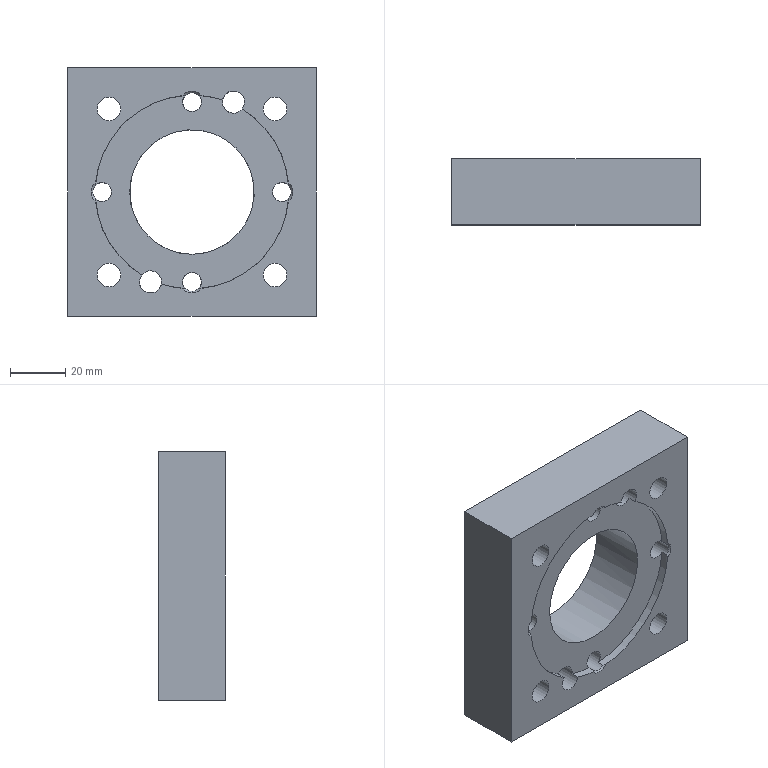Part | STEP file | 冲床-300配套压波_id958_x_t | 1 solid | 40 faces | box 90 x 24 x 90 mm | volume 133155 mm3 | cylinder 21 | plane 11 | cone 8 | commonest cylinder face diameters 70 x6 6.8 x4 8.5 x4 14 x4 8 x2 45 x1
STEP:
#1=CARTESIAN_POINT('',(1380.937,43.5,46.878));
#2=VERTEX_POINT('',#1);
#3=CARTESIAN_POINT('',(1380.937,46.5,46.878));
#4=VERTEX_POINT('',#3);
#5=CARTESIAN_POINT('',(1380.937,20.,46.878));
#6=DIRECTION('',(0.,1.,0.));
#7=VECTOR('',#6,1.);
#8=LINE('',#5,#7);
#9=EDGE_CURVE('',#2,#4,#8,.T.);
#10=ORIENTED_EDGE('',*,*,#9,.F.);
#11=CARTESIAN_POINT('',(1388.763,43.5,45.233));
#12=VERTEX_POINT('',#11);
#13=CARTESIAN_POINT('',(1392.,43.5,80.083));
#14=DIRECTION('',(0.,-1.,0.));
#15=DIRECTION('',(0.,0.,-1.));
#16=AXIS2_PLACEMENT_3D('',#13,#14,#15);
#17=CIRCLE('',#16,35.);
#18=EDGE_CURVE('',#2,#12,#17,.T.);
#19=ORIENTED_EDGE('',*,*,#18,.T.);
#20=CARTESIAN_POINT('',(1389.61,44.1,45.165));
#21=VERTEX_POINT('',#20);
#22=CARTESIAN_POINT('',(1388.763,43.5,45.233));
#23=CARTESIAN_POINT('',(1389.039,43.708,45.208));
#24=CARTESIAN_POINT('',(1389.32,43.91,45.185));
#25=CARTESIAN_POINT('',(1389.61,44.1,45.165));
#26=B_SPLINE_CURVE_WITH_KNOTS('',3,(#22,#23,#24,#25),.UNSPECIFIED.,.F.,.F.,(4,4),(0.,1.),.UNSPECIFIED.);
#27=EDGE_CURVE('',#12,#21,#26,.T.);
#28=ORIENTED_EDGE('',*,*,#27,.T.);
#29=CARTESIAN_POINT('',(1389.61,46.5,45.165));
#30=VERTEX_POINT('',#29);
#31=CARTESIAN_POINT('',(1389.61,-247465.249,45.165));
#32=DIRECTION('',(0.,1.,0.));
#33=VECTOR('',#32,1.);
#34=LINE('',#31,#33);
#35=EDGE_CURVE('',#21,#30,#34,.T.);
#36=ORIENTED_EDGE('',*,*,#35,.T.);
#37=CARTESIAN_POINT('',(1392.,46.5,80.083));
#38=DIRECTION('',(0.,1.,0.));
#39=DIRECTION('',(-1.,0.,0.));
#40=AXIS2_PLACEMENT_3D('',#37,#38,#39);
#41=CIRCLE('',#40,35.);
#42=EDGE_CURVE('',#30,#4,#41,.T.);
#43=ORIENTED_EDGE('',*,*,#42,.T.);
#44=EDGE_LOOP('',(#10,#19,#28,#36,#43));
#45=FACE_OUTER_BOUND('',#44,.T.);
#46=CARTESIAN_POINT('',(1392.,-46.,80.083));
#47=DIRECTION('',(0.,-1.,0.));
#48=DIRECTION('',(0.,0.,-1.));
#49=AXIS2_PLACEMENT_3D('',#46,#47,#48);
#50=CYLINDRICAL_SURFACE('',#49,35.);
#51=ADVANCED_FACE('',(#45),#50,.F.);
#52=CARTESIAN_POINT('',(1373.909,46.5,50.122));
#53=VERTEX_POINT('',#52);
#54=CARTESIAN_POINT('',(1373.909,43.5,50.122));
#55=VERTEX_POINT('',#54);
#56=CARTESIAN_POINT('',(1373.909,20.,50.122));
#57=DIRECTION('',(0.,-1.,0.));
#58=VECTOR('',#57,1.);
#59=LINE('',#56,#58);
#60=EDGE_CURVE('',#53,#55,#59,.T.);
#61=ORIENTED_EDGE('',*,*,#60,.F.);
#62=CARTESIAN_POINT('',(1357.082,46.5,77.694));
#63=VERTEX_POINT('',#62);
#64=CARTESIAN_POINT('',(1392.,46.5,80.083));
#65=DIRECTION('',(0.,1.,0.));
#66=DIRECTION('',(-1.,0.,0.));
#67=AXIS2_PLACEMENT_3D('',#64,#65,#66);
#68=CIRCLE('',#67,35.);
#69=EDGE_CURVE('',#53,#63,#68,.T.);
#70=ORIENTED_EDGE('',*,*,#69,.T.);
#71=CARTESIAN_POINT('',(1357.082,44.1,77.694));
#72=VERTEX_POINT('',#71);
#73=CARTESIAN_POINT('',(1357.082,-247465.293,77.694));
#74=DIRECTION('',(0.,-1.,0.));
#75=VECTOR('',#74,1.);
#76=LINE('',#73,#75);
#77=EDGE_CURVE('',#63,#72,#76,.T.);
#78=ORIENTED_EDGE('',*,*,#77,.T.);
#79=CARTESIAN_POINT('',(1357.15,43.5,76.847));
#80=VERTEX_POINT('',#79);
#81=CARTESIAN_POINT('',(1357.082,44.1,77.694));
#82=CARTESIAN_POINT('',(1357.102,43.91,77.404));
#83=CARTESIAN_POINT('',(1357.124,43.708,77.123));
#84=CARTESIAN_POINT('',(1357.15,43.5,76.847));
#85=B_SPLINE_CURVE_WITH_KNOTS('',3,(#81,#82,#83,#84),.UNSPECIFIED.,.F.,.F.,(4,4),(0.,1.),.UNSPECIFIED.);
#86=EDGE_CURVE('',#72,#80,#85,.T.);
#87=ORIENTED_EDGE('',*,*,#86,.T.);
#88=CARTESIAN_POINT('',(1392.,43.5,80.083));
#89=DIRECTION('',(0.,-1.,0.));
#90=DIRECTION('',(0.,0.,-1.));
#91=AXIS2_PLACEMENT_3D('',#88,#89,#90);
#92=CIRCLE('',#91,35.);
#93=EDGE_CURVE('',#80,#55,#92,.T.);
#94=ORIENTED_EDGE('',*,*,#93,.T.);
#95=EDGE_LOOP('',(#61,#70,#78,#87,#94));
#96=FACE_OUTER_BOUND('',#95,.T.);
#97=CARTESIAN_POINT('',(1392.,-46.,80.083));
#98=DIRECTION('',(0.,-1.,0.));
#99=DIRECTION('',(0.,0.,-1.));
#100=AXIS2_PLACEMENT_3D('',#97,#98,#99);
#101=CYLINDRICAL_SURFACE('',#100,35.);
#102=ADVANCED_FACE('',(#96),#101,.F.);
#103=CARTESIAN_POINT('',(1403.063,43.5,113.289));
#104=VERTEX_POINT('',#103);
#105=CARTESIAN_POINT('',(1403.063,46.5,113.289));
#106=VERTEX_POINT('',#105);
#107=CARTESIAN_POINT('',(1403.063,20.,113.289));
#108=DIRECTION('',(0.,1.,0.));
#109=VECTOR('',#108,1.);
#110=LINE('',#107,#109);
#111=EDGE_CURVE('',#104,#106,#110,.T.);
#112=ORIENTED_EDGE('',*,*,#111,.F.);
#113=CARTESIAN_POINT('',(1395.237,43.5,114.933));
#114=VERTEX_POINT('',#113);
#115=CARTESIAN_POINT('',(1392.,43.5,80.083));
#116=DIRECTION('',(0.,-1.,0.));
#117=DIRECTION('',(0.,0.,-1.));
#118=AXIS2_PLACEMENT_3D('',#115,#116,#117);
#119=CIRCLE('',#118,35.);
#120=EDGE_CURVE('',#104,#114,#119,.T.);
#121=ORIENTED_EDGE('',*,*,#120,.T.);
#122=CARTESIAN_POINT('',(1394.39,44.1,115.002));
#123=VERTEX_POINT('',#122);
#124=CARTESIAN_POINT('',(1395.237,43.5,114.933));
#125=CARTESIAN_POINT('',(1394.961,43.708,114.959));
#126=CARTESIAN_POINT('',(1394.68,43.91,114.982));
#127=CARTESIAN_POINT('',(1394.39,44.1,115.002));
#128=B_SPLINE_CURVE_WITH_KNOTS('',3,(#124,#125,#126,#127),.UNSPECIFIED.,.F.,.F.,(4,4),(0.,1.),.UNSPECIFIED.);
#129=EDGE_CURVE('',#114,#123,#128,.T.);
#130=ORIENTED_EDGE('',*,*,#129,.T.);
#131=CARTESIAN_POINT('',(1394.39,46.5,115.002));
#132=VERTEX_POINT('',#131);
#133=CARTESIAN_POINT('',(1394.39,-247465.244,115.002));
#134=DIRECTION('',(0.,1.,0.));
#135=VECTOR('',#134,1.);
#136=LINE('',#133,#135);
#137=EDGE_CURVE('',#123,#132,#136,.T.);
#138=ORIENTED_EDGE('',*,*,#137,.T.);
#139=CARTESIAN_POINT('',(1392.,46.5,80.083));
#140=DIRECTION('',(0.,1.,0.));
#141=DIRECTION('',(-1.,0.,0.));
#142=AXIS2_PLACEMENT_3D('',#139,#140,#141);
#143=CIRCLE('',#142,35.);
#144=EDGE_CURVE('',#132,#106,#143,.T.);
#145=ORIENTED_EDGE('',*,*,#144,.T.);
#146=EDGE_LOOP('',(#112,#121,#130,#138,#145));
#147=FACE_OUTER_BOUND('',#146,.T.);
#148=CARTESIAN_POINT('',(1392.,-46.,80.083));
#149=DIRECTION('',(0.,-1.,0.));
#150=DIRECTION('',(0.,0.,-1.));
#151=AXIS2_PLACEMENT_3D('',#148,#149,#150);
#152=CYLINDRICAL_SURFACE('',#151,35.);
#153=ADVANCED_FACE('',(#147),#152,.F.);
#154=CARTESIAN_POINT('',(1410.091,46.5,110.045));
#155=VERTEX_POINT('',#154);
#156=CARTESIAN_POINT('',(1410.091,43.5,110.045));
#157=VERTEX_POINT('',#156);
#158=CARTESIAN_POINT('',(1410.091,20.,110.045));
#159=DIRECTION('',(0.,-1.,0.));
#160=VECTOR('',#159,1.);
#161=LINE('',#158,#160);
#162=EDGE_CURVE('',#155,#157,#161,.T.);
#163=ORIENTED_EDGE('',*,*,#162,.F.);
#164=CARTESIAN_POINT('',(1426.918,46.5,82.473));
#165=VERTEX_POINT('',#164);
#166=CARTESIAN_POINT('',(1392.,46.5,80.083));
#167=DIRECTION('',(0.,1.,0.));
#168=DIRECTION('',(-1.,0.,0.));
#169=AXIS2_PLACEMENT_3D('',#166,#167,#168);
#170=CIRCLE('',#169,35.);
#171=EDGE_CURVE('',#155,#165,#170,.T.);
#172=ORIENTED_EDGE('',*,*,#171,.T.);
#173=CARTESIAN_POINT('',(1426.918,44.1,82.473));
#174=VERTEX_POINT('',#173);
#175=CARTESIAN_POINT('',(1426.918,-247465.2,82.473));
#176=DIRECTION('',(0.,-1.,0.));
#177=VECTOR('',#176,1.);
#178=LINE('',#175,#177);
#179=EDGE_CURVE('',#165,#174,#178,.T.);
#180=ORIENTED_EDGE('',*,*,#179,.T.);
#181=CARTESIAN_POINT('',(1426.85,43.5,83.32));
#182=VERTEX_POINT('',#181);
#183=CARTESIAN_POINT('',(1426.918,44.1,82.473));
#184=CARTESIAN_POINT('',(1426.898,43.91,82.763));
#185=CARTESIAN_POINT('',(1426.876,43.708,83.044));
#186=CARTESIAN_POINT('',(1426.85,43.5,83.32));
#187=B_SPLINE_CURVE_WITH_KNOTS('',3,(#183,#184,#185,#186),.UNSPECIFIED.,.F.,.F.,(4,4),(0.,1.),.UNSPECIFIED.);
#188=EDGE_CURVE('',#174,#182,#187,.T.);
#189=ORIENTED_EDGE('',*,*,#188,.T.);
#190=CARTESIAN_POINT('',(1392.,43.5,80.083));
#191=DIRECTION('',(0.,-1.,0.));
#192=DIRECTION('',(0.,0.,-1.));
#193=AXIS2_PLACEMENT_3D('',#190,#191,#192);
#194=CIRCLE('',#193,35.);
#195=EDGE_CURVE('',#182,#157,#194,.T.);
#196=ORIENTED_EDGE('',*,*,#195,.T.);
#197=EDGE_LOOP('',(#163,#172,#180,#189,#196));
#198=FACE_OUTER_BOUND('',#197,.T.);
#199=CARTESIAN_POINT('',(1392.,-46.,80.083));
#200=DIRECTION('',(0.,-1.,0.));
#201=DIRECTION('',(0.,0.,-1.));
#202=AXIS2_PLACEMENT_3D('',#199,#200,#201);
#203=CYLINDRICAL_SURFACE('',#202,35.);
#204=ADVANCED_FACE('',(#198),#203,.F.);
#205=CARTESIAN_POINT('',(1357.082,44.1,82.473));
#206=VERTEX_POINT('',#205);
#207=CARTESIAN_POINT('',(1357.082,46.5,82.473));
#208=VERTEX_POINT('',#207);
#209=CARTESIAN_POINT('',(1357.082,-247465.293,82.473));
#210=DIRECTION('',(0.,1.,0.));
#211=VECTOR('',#210,1.);
#212=LINE('',#209,#211);
#213=EDGE_CURVE('',#206,#208,#212,.T.);
#214=ORIENTED_EDGE('',*,*,#213,.T.);
#215=CARTESIAN_POINT('',(1389.61,46.5,115.002));
#216=VERTEX_POINT('',#215);
#217=CARTESIAN_POINT('',(1392.,46.5,80.083));
#218=DIRECTION('',(0.,1.,0.));
#219=DIRECTION('',(-1.,0.,0.));
#220=AXIS2_PLACEMENT_3D('',#217,#218,#219);
#221=CIRCLE('',#220,35.);
#222=EDGE_CURVE('',#208,#216,#221,.T.);
#223=ORIENTED_EDGE('',*,*,#222,.T.);
#224=CARTESIAN_POINT('',(1389.61,44.1,115.002));
#225=VERTEX_POINT('',#224);
#226=CARTESIAN_POINT('',(1389.61,-247465.244,115.002));
#227=DIRECTION('',(0.,-1.,0.));
#228=VECTOR('',#227,1.);
#229=LINE('',#226,#228);
#230=EDGE_CURVE('',#216,#225,#229,.T.);
#231=ORIENTED_EDGE('',*,*,#230,.T.);
#232=CARTESIAN_POINT('',(1388.763,43.5,114.933));
#233=VERTEX_POINT('',#232);
#234=CARTESIAN_POINT('',(1389.61,44.1,115.002));
#235=CARTESIAN_POINT('',(1389.32,43.91,114.982));
#236=CARTESIAN_POINT('',(1389.039,43.708,114.959));
#237=CARTESIAN_POINT('',(1388.763,43.5,114.933));
#238=B_SPLINE_CURVE_WITH_KNOTS('',3,(#234,#235,#236,#237),.UNSPECIFIED.,.F.,.F.,(4,4),(0.,1.),.UNSPECIFIED.);
#239=EDGE_CURVE('',#225,#233,#238,.T.);
#240=ORIENTED_EDGE('',*,*,#239,.T.);
#241=CARTESIAN_POINT('',(1357.15,43.5,83.32));
#242=VERTEX_POINT('',#241);
#243=CARTESIAN_POINT('',(1392.,43.5,80.083));
#244=DIRECTION('',(0.,-1.,0.));
#245=DIRECTION('',(0.,0.,-1.));
#246=AXIS2_PLACEMENT_3D('',#243,#244,#245);
#247=CIRCLE('',#246,35.);
#248=EDGE_CURVE('',#233,#242,#247,.T.);
#249=ORIENTED_EDGE('',*,*,#248,.T.);
#250=CARTESIAN_POINT('',(1357.15,43.5,83.32));
#251=CARTESIAN_POINT('',(1357.124,43.708,83.044));
#252=CARTESIAN_POINT('',(1357.102,43.91,82.763));
#253=CARTESIAN_POINT('',(1357.082,44.1,82.473));
#254=B_SPLINE_CURVE_WITH_KNOTS('',3,(#250,#251,#252,#253),.UNSPECIFIED.,.F.,.F.,(4,4),(0.,1.),.UNSPECIFIED.);
#255=EDGE_CURVE('',#242,#206,#254,.T.);
#256=ORIENTED_EDGE('',*,*,#255,.T.);
#257=EDGE_LOOP('',(#214,#223,#231,#240,#249,#256));
#258=FACE_OUTER_BOUND('',#257,.T.);
#259=CARTESIAN_POINT('',(1392.,-46.,80.083));
#260=DIRECTION('',(0.,-1.,0.));
#261=DIRECTION('',(0.,0.,-1.));
#262=AXIS2_PLACEMENT_3D('',#259,#260,#261);
#263=CYLINDRICAL_SURFACE('',#262,35.);
#264=ADVANCED_FACE('',(#258),#263,.F.);
#265=CARTESIAN_POINT('',(1395.237,43.5,45.233));
#266=VERTEX_POINT('',#265);
#267=CARTESIAN_POINT('',(1426.85,43.5,76.847));
#268=VERTEX_POINT('',#267);
#269=CARTESIAN_POINT('',(1392.,43.5,80.083));
#270=DIRECTION('',(0.,-1.,0.));
#271=DIRECTION('',(0.,0.,-1.));
#272=AXIS2_PLACEMENT_3D('',#269,#270,#271);
#273=CIRCLE('',#272,35.);
#274=EDGE_CURVE('',#266,#268,#273,.T.);
#275=ORIENTED_EDGE('',*,*,#274,.T.);
#276=CARTESIAN_POINT('',(1426.918,44.1,77.694));
#277=VERTEX_POINT('',#276);
#278=CARTESIAN_POINT('',(1426.85,43.5,76.847));
#279=CARTESIAN_POINT('',(1426.876,43.708,77.123));
#280=CARTESIAN_POINT('',(1426.898,43.91,77.404));
#281=CARTESIAN_POINT('',(1426.918,44.1,77.694));
#282=B_SPLINE_CURVE_WITH_KNOTS('',3,(#278,#279,#280,#281),.UNSPECIFIED.,.F.,.F.,(4,4),(0.,1.),.UNSPECIFIED.);
#283=EDGE_CURVE('',#268,#277,#282,.T.);
#284=ORIENTED_EDGE('',*,*,#283,.T.);
#285=CARTESIAN_POINT('',(1426.918,46.5,77.694));
#286=VERTEX_POINT('',#285);
#287=CARTESIAN_POINT('',(1426.918,-247465.2,77.694));
#288=DIRECTION('',(0.,1.,0.));
#289=VECTOR('',#288,1.);
#290=LINE('',#287,#289);
#291=EDGE_CURVE('',#277,#286,#290,.T.);
#292=ORIENTED_EDGE('',*,*,#291,.T.);
#293=CARTESIAN_POINT('',(1394.39,46.5,45.165));
#294=VERTEX_POINT('',#293);
#295=CARTESIAN_POINT('',(1392.,46.5,80.083));
#296=DIRECTION('',(0.,1.,0.));
#297=DIRECTION('',(-1.,0.,0.));
#298=AXIS2_PLACEMENT_3D('',#295,#296,#297);
#299=CIRCLE('',#298,35.);
#300=EDGE_CURVE('',#286,#294,#299,.T.);
#301=ORIENTED_EDGE('',*,*,#300,.T.);
#302=CARTESIAN_POINT('',(1394.39,44.1,45.165));
#303=VERTEX_POINT('',#302);
#304=CARTESIAN_POINT('',(1394.39,-247465.249,45.165));
#305=DIRECTION('',(0.,-1.,0.));
#306=VECTOR('',#305,1.);
#307=LINE('',#304,#306);
#308=EDGE_CURVE('',#294,#303,#307,.T.);
#309=ORIENTED_EDGE('',*,*,#308,.T.);
#310=CARTESIAN_POINT('',(1394.39,44.1,45.165));
#311=CARTESIAN_POINT('',(1394.68,43.91,45.185));
#312=CARTESIAN_POINT('',(1394.961,43.708,45.208));
#313=CARTESIAN_POINT('',(1395.237,43.5,45.233));
#314=B_SPLINE_CURVE_WITH_KNOTS('',3,(#310,#311,#312,#313),.UNSPECIFIED.,.F.,.F.,(4,4),(0.,1.),.UNSPECIFIED.);
#315=EDGE_CURVE('',#303,#266,#314,.T.);
#316=ORIENTED_EDGE('',*,*,#315,.T.);
#317=EDGE_LOOP('',(#275,#284,#292,#301,#309,#316));
#318=FACE_OUTER_BOUND('',#317,.T.);
#319=CARTESIAN_POINT('',(1392.,-46.,80.083));
#320=DIRECTION('',(0.,-1.,0.));
#321=DIRECTION('',(0.,0.,-1.));
#322=AXIS2_PLACEMENT_3D('',#319,#320,#321);
#323=CYLINDRICAL_SURFACE('',#322,35.);
#324=ADVANCED_FACE('',(#318),#323,.F.);
#325=CARTESIAN_POINT('',(1403.,67.5,112.583));
#326=VERTEX_POINT('',#325);
#327=CARTESIAN_POINT('',(1407.,67.5,112.583));
#328=DIRECTION('',(0.,-1.,0.));
#329=DIRECTION('',(-1.,0.,0.));
#330=AXIS2_PLACEMENT_3D('',#327,#328,#329);
#331=CIRCLE('',#330,4.);
#332=EDGE_CURVE('',#326,#326,#331,.T.);
#333=ORIENTED_EDGE('',*,*,#332,.T.);
#334=EDGE_LOOP('',(#333));
#335=FACE_BOUND('',#334,.T.);
#336=CARTESIAN_POINT('',(1373.,67.5,47.583));
#337=VERTEX_POINT('',#336);
#338=CARTESIAN_POINT('',(1377.,67.5,47.583));
#339=DIRECTION('',(0.,-1.,0.));
#340=DIRECTION('',(-1.,0.,0.));
#341=AXIS2_PLACEMENT_3D('',#338,#339,#340);
#342=CIRCLE('',#341,4.);
#343=EDGE_CURVE('',#337,#337,#342,.T.);
#344=ORIENTED_EDGE('',*,*,#343,.T.);
#345=EDGE_LOOP('',(#344));
#346=FACE_BOUND('',#345,.T.);
#347=CARTESIAN_POINT('',(1392.,67.5,43.583));
#348=VERTEX_POINT('',#347);
#349=CARTESIAN_POINT('',(1392.,67.5,47.583));
#350=DIRECTION('',(0.,-1.,0.));
#351=DIRECTION('',(0.,0.,-1.));
#352=AXIS2_PLACEMENT_3D('',#349,#350,#351);
#353=CIRCLE('',#352,4.);
#354=EDGE_CURVE('',#348,#348,#353,.T.);
#355=ORIENTED_EDGE('',*,*,#354,.T.);
#356=EDGE_LOOP('',(#355));
#357=FACE_BOUND('',#356,.T.);
#358=CARTESIAN_POINT('',(1424.5,67.5,76.083));
#359=VERTEX_POINT('',#358);
#360=CARTESIAN_POINT('',(1424.5,67.5,80.083));
#361=DIRECTION('',(0.,-1.,0.));
#362=DIRECTION('',(0.,0.,-1.));
#363=AXIS2_PLACEMENT_3D('',#360,#361,#362);
#364=CIRCLE('',#363,4.);
#365=EDGE_CURVE('',#359,#359,#364,.T.);
#366=ORIENTED_EDGE('',*,*,#365,.T.);
#367=EDGE_LOOP('',(#366));
#368=FACE_BOUND('',#367,.T.);
#369=CARTESIAN_POINT('',(1359.5,67.5,76.083));
#370=VERTEX_POINT('',#369);
#371=CARTESIAN_POINT('',(1359.5,67.5,80.083));
#372=DIRECTION('',(0.,-1.,0.));
#373=DIRECTION('',(0.,0.,-1.));
#374=AXIS2_PLACEMENT_3D('',#371,#372,#373);
#375=CIRCLE('',#374,4.);
#376=EDGE_CURVE('',#370,#370,#375,.T.);
#377=ORIENTED_EDGE('',*,*,#376,.T.);
#378=EDGE_LOOP('',(#377));
#379=FACE_BOUND('',#378,.T.);
#380=CARTESIAN_POINT('',(1392.,67.5,108.583));
#381=VERTEX_POINT('',#380);
#382=CARTESIAN_POINT('',(1392.,67.5,112.583));
#383=DIRECTION('',(0.,-1.,0.));
#384=DIRECTION('',(0.,0.,-1.));
#385=AXIS2_PLACEMENT_3D('',#382,#383,#384);
#386=CIRCLE('',#385,4.);
#387=EDGE_CURVE('',#381,#381,#386,.T.);
#388=ORIENTED_EDGE('',*,*,#387,.T.);
#389=EDGE_LOOP('',(#388));
#390=FACE_BOUND('',#389,.T.);
#391=CARTESIAN_POINT('',(1392.,67.5,57.583));
#392=VERTEX_POINT('',#391);
#393=CARTESIAN_POINT('',(1392.,67.5,80.083));
#394=DIRECTION('',(0.,1.,0.));
#395=DIRECTION('',(0.,0.,-1.));
#396=AXIS2_PLACEMENT_3D('',#393,#394,#395);
#397=CIRCLE('',#396,22.5);
#398=EDGE_CURVE('',#392,#392,#397,.T.);
#399=ORIENTED_EDGE('',*,*,#398,.F.);
#400=EDGE_LOOP('',(#399));
#401=FACE_BOUND('',#400,.T.);
#402=CARTESIAN_POINT('',(1422.052,67.5,103.136));
#403=VERTEX_POINT('',#402);
#404=CARTESIAN_POINT('',(1422.052,67.5,110.136));
#405=DIRECTION('',(0.,1.,0.));
#406=DIRECTION('',(0.,0.,-1.));
#407=AXIS2_PLACEMENT_3D('',#404,#405,#406);
#408=CIRCLE('',#407,7.);
#409=EDGE_CURVE('',#403,#403,#408,.T.);
#410=ORIENTED_EDGE('',*,*,#409,.F.);
#411=EDGE_LOOP('',(#410));
#412=FACE_BOUND('',#411,.T.);
#413=CARTESIAN_POINT('',(1361.948,67.5,43.031));
#414=VERTEX_POINT('',#413);
#415=CARTESIAN_POINT('',(1361.948,67.5,50.031));
#416=DIRECTION('',(0.,1.,0.));
#417=DIRECTION('',(0.,0.,-1.));
#418=AXIS2_PLACEMENT_3D('',#415,#416,#417);
#419=CIRCLE('',#418,7.);
#420=EDGE_CURVE('',#414,#414,#419,.T.);
#421=ORIENTED_EDGE('',*,*,#420,.F.);
#422=EDGE_LOOP('',(#421));
#423=FACE_BOUND('',#422,.T.);
#424=CARTESIAN_POINT('',(1422.052,67.5,43.031));
#425=VERTEX_POINT('',#424);
#426=CARTESIAN_POINT('',(1422.052,67.5,50.031));
#427=DIRECTION('',(0.,1.,0.));
#428=DIRECTION('',(0.,0.,-1.));
#429=AXIS2_PLACEMENT_3D('',#426,#427,#428);
#430=CIRCLE('',#429,7.);
#431=EDGE_CURVE('',#425,#425,#430,.T.);
#432=ORIENTED_EDGE('',*,*,#431,.F.);
#433=EDGE_LOOP('',(#432));
#434=FACE_BOUND('',#433,.T.);
#435=CARTESIAN_POINT('',(1361.948,67.5,103.136));
#436=VERTEX_POINT('',#435);
#437=CARTESIAN_POINT('',(1361.948,67.5,110.136));
#438=DIRECTION('',(0.,-1.,0.));
#439=DIRECTION('',(0.,0.,-1.));
#440=AXIS2_PLACEMENT_3D('',#437,#438,#439);
#441=CIRCLE('',#440,7.);
#442=EDGE_CURVE('',#436,#436,#441,.T.);
#443=ORIENTED_EDGE('',*,*,#442,.T.);
#444=EDGE_LOOP('',(#443));
#445=FACE_BOUND('',#444,.T.);
#446=CARTESIAN_POINT('',(1347.,67.5,35.083));
#447=VERTEX_POINT('',#446);
#448=CARTESIAN_POINT('',(1347.,67.5,125.083));
#449=VERTEX_POINT('',#448);
#450=CARTESIAN_POINT('',(1347.,67.5,24.7));
#451=DIRECTION('',(0.,0.,1.));
#452=VECTOR('',#451,1.);
#453=LINE('',#450,#452);
#454=EDGE_CURVE('',#447,#449,#453,.T.);
#455=ORIENTED_EDGE('',*,*,#454,.T.);
#456=CARTESIAN_POINT('',(1437.,67.5,125.083));
#457=VERTEX_POINT('',#456);
#458=CARTESIAN_POINT('',(1437.,67.5,125.083));
#459=DIRECTION('',(1.,0.,0.));
#460=VECTOR('',#459,1.);
#461=LINE('',#458,#460);
#462=EDGE_CURVE('',#449,#457,#461,.T.);
#463=ORIENTED_EDGE('',*,*,#462,.T.);
#464=CARTESIAN_POINT('',(1437.,67.5,35.083));
#465=VERTEX_POINT('',#464);
#466=CARTESIAN_POINT('',(1437.,67.5,35.083));
#467=DIRECTION('',(0.,0.,-1.));
#468=VECTOR('',#467,1.);
#469=LINE('',#466,#468);
#470=EDGE_CURVE('',#457,#465,#469,.T.);
#471=ORIENTED_EDGE('',*,*,#470,.T.);
#472=CARTESIAN_POINT('',(1347.,67.5,35.083));
#473=DIRECTION('',(-1.,0.,0.));
#474=VECTOR('',#473,1.);
#475=LINE('',#472,#474);
#476=EDGE_CURVE('',#465,#447,#475,.T.);
#477=ORIENTED_EDGE('',*,*,#476,.T.);
#478=EDGE_LOOP('',(#455,#463,#471,#477));
#479=FACE_BOUND('',#478,.T.);
#480=CARTESIAN_POINT('',(-14.812,67.5,1.089));
#481=DIRECTION('',(0.,1.,0.));
#482=DIRECTION('',(0.,0.,-1.));
#483=AXIS2_PLACEMENT_3D('',#480,#481,#482);
#484=PLANE('',#483);
#485=ADVANCED_FACE('',(#335,#346,#357,#368,#379,#390,#401,#412,#423,#434,#445,#479),#484,.T.);
#486=CARTESIAN_POINT('',(1361.948,43.5,45.781));
#487=VERTEX_POINT('',#486);
#488=CARTESIAN_POINT('',(1361.948,43.5,50.031));
#489=DIRECTION('',(0.,1.,0.));
#490=DIRECTION('',(0.,0.,-1.));
#491=AXIS2_PLACEMENT_3D('',#488,#489,#490);
#492=CIRCLE('',#491,4.25);
#493=EDGE_CURVE('',#487,#487,#492,.T.);
#494=ORIENTED_EDGE('',*,*,#493,.F.);
#495=EDGE_LOOP('',(#494));
#496=FACE_BOUND('',#495,.T.);
#497=CARTESIAN_POINT('',(1361.948,53.5,45.781));
#498=VERTEX_POINT('',#497);
#499=CARTESIAN_POINT('',(1361.948,53.5,50.031));
#500=DIRECTION('',(0.,-1.,0.));
#501=DIRECTION('',(0.,0.,-1.));
#502=AXIS2_PLACEMENT_3D('',#499,#500,#501);
#503=CIRCLE('',#502,4.25);
#504=EDGE_CURVE('',#498,#498,#503,.T.);
#505=ORIENTED_EDGE('',*,*,#504,.F.);
#506=EDGE_LOOP('',(#505));
#507=FACE_BOUND('',#506,.T.);
#508=CARTESIAN_POINT('',(1361.948,23.5,50.031));
#509=DIRECTION('',(0.,1.,0.));
#510=DIRECTION('',(1.,0.,0.));
#511=AXIS2_PLACEMENT_3D('',#508,#509,#510);
#512=CYLINDRICAL_SURFACE('',#511,4.25);
#513=ADVANCED_FACE('',(#496,#507),#512,.F.);
#514=CARTESIAN_POINT('',(1422.052,43.5,105.886));
#515=VERTEX_POINT('',#514);
#516=CARTESIAN_POINT('',(1422.052,43.5,110.136));
#517=DIRECTION('',(0.,1.,0.));
#518=DIRECTION('',(0.,0.,-1.));
#519=AXIS2_PLACEMENT_3D('',#516,#517,#518);
#520=CIRCLE('',#519,4.25);
#521=EDGE_CURVE('',#515,#515,#520,.T.);
#522=ORIENTED_EDGE('',*,*,#521,.F.);
#523=EDGE_LOOP('',(#522));
#524=FACE_BOUND('',#523,.T.);
#525=CARTESIAN_POINT('',(1422.052,53.5,105.886));
#526=VERTEX_POINT('',#525);
#527=CARTESIAN_POINT('',(1422.052,53.5,110.136));
#528=DIRECTION('',(0.,-1.,0.));
#529=DIRECTION('',(0.,0.,-1.));
#530=AXIS2_PLACEMENT_3D('',#527,#528,#529);
#531=CIRCLE('',#530,4.25);
#532=EDGE_CURVE('',#526,#526,#531,.T.);
#533=ORIENTED_EDGE('',*,*,#532,.F.);
#534=EDGE_LOOP('',(#533));
#535=FACE_BOUND('',#534,.T.);
#536=CARTESIAN_POINT('',(1422.052,23.5,110.136));
#537=DIRECTION('',(0.,1.,0.));
#538=DIRECTION('',(1.,0.,0.));
#539=AXIS2_PLACEMENT_3D('',#536,#537,#538);
#540=CYLINDRICAL_SURFACE('',#539,4.25);
#541=ADVANCED_FACE('',(#524,#535),#540,.F.);
#542=CARTESIAN_POINT('',(1422.052,43.5,45.781));
#543=VERTEX_POINT('',#542);
#544=CARTESIAN_POINT('',(1422.052,43.5,50.031));
#545=DIRECTION('',(0.,1.,0.));
#546=DIRECTION('',(0.,0.,-1.));
#547=AXIS2_PLACEMENT_3D('',#544,#545,#546);
#548=CIRCLE('',#547,4.25);
#549=EDGE_CURVE('',#543,#543,#548,.T.);
#550=ORIENTED_EDGE('',*,*,#549,.F.);
#551=EDGE_LOOP('',(#550));
#552=FACE_BOUND('',#551,.T.);
#553=CARTESIAN_POINT('',(1422.052,53.5,45.781));
#554=VERTEX_POINT('',#553);
#555=CARTESIAN_POINT('',(1422.052,53.5,50.031));
#556=DIRECTION('',(0.,-1.,0.));
#557=DIRECTION('',(0.,0.,-1.));
#558=AXIS2_PLACEMENT_3D('',#555,#556,#557);
#559=CIRCLE('',#558,4.25);
#560=EDGE_CURVE('',#554,#554,#559,.T.);
#561=ORIENTED_EDGE('',*,*,#560,.F.);
#562=EDGE_LOOP('',(#561));
#563=FACE_BOUND('',#562,.T.);
#564=CARTESIAN_POINT('',(1422.052,23.5,50.031));
#565=DIRECTION('',(0.,1.,0.));
#566=DIRECTION('',(1.,0.,0.));
#567=AXIS2_PLACEMENT_3D('',#564,#565,#566);
#568=CYLINDRICAL_SURFACE('',#567,4.25);
#569=ADVANCED_FACE('',(#552,#563),#568,.F.);
#570=CARTESIAN_POINT('',(1407.,43.5,112.583));
#571=DIRECTION('',(0.,-1.,0.));
#572=DIRECTION('',(-1.,0.,0.));
#573=AXIS2_PLACEMENT_3D('',#570,#571,#572);
#574=CIRCLE('',#573,4.);
#575=EDGE_CURVE('',#157,#104,#574,.T.);
#576=ORIENTED_EDGE('',*,*,#575,.F.);
#577=ORIENTED_EDGE('',*,*,#195,.F.);
#578=CARTESIAN_POINT('',(1424.5,43.5,80.083));
#579=DIRECTION('',(0.,1.,0.));
#580=DIRECTION('',(0.,0.,-1.));
#581=AXIS2_PLACEMENT_3D('',#578,#579,#580);
#582=CIRCLE('',#581,4.);
#583=EDGE_CURVE('',#182,#268,#582,.T.);
#584=ORIENTED_EDGE('',*,*,#583,.T.);
#585=ORIENTED_EDGE('',*,*,#274,.F.);
#586=CARTESIAN_POINT('',(1392.,43.5,47.583));
#587=DIRECTION('',(0.,1.,0.));
#588=DIRECTION('',(0.,0.,-1.));
#589=AXIS2_PLACEMENT_3D('',#586,#587,#588);
#590=CIRCLE('',#589,4.);
#591=EDGE_CURVE('',#266,#12,#590,.T.);
#592=ORIENTED_EDGE('',*,*,#591,.T.);
#593=ORIENTED_EDGE('',*,*,#18,.F.);
#594=CARTESIAN_POINT('',(1377.,43.5,47.583));
#595=DIRECTION('',(0.,-1.,0.));
#596=DIRECTION('',(-1.,0.,0.));
#597=AXIS2_PLACEMENT_3D('',#594,#595,#596);
#598=CIRCLE('',#597,4.);
#599=EDGE_CURVE('',#55,#2,#598,.T.);
#600=ORIENTED_EDGE('',*,*,#599,.F.);
#601=ORIENTED_EDGE('',*,*,#93,.F.);
#602=CARTESIAN_POINT('',(1359.5,43.5,80.083));
#603=DIRECTION('',(0.,1.,0.));
#604=DIRECTION('',(0.,0.,-1.));
#605=AXIS2_PLACEMENT_3D('',#602,#603,#604);
#606=CIRCLE('',#605,4.);
#607=EDGE_CURVE('',#80,#242,#606,.T.);
#608=ORIENTED_EDGE('',*,*,#607,.T.);
#609=ORIENTED_EDGE('',*,*,#248,.F.);
#610=CARTESIAN_POINT('',(1392.,43.5,112.583));
#611=DIRECTION('',(0.,1.,0.));
#612=DIRECTION('',(0.,0.,-1.));
#613=AXIS2_PLACEMENT_3D('',#610,#611,#612);
#614=CIRCLE('',#613,4.);
#615=EDGE_CURVE('',#233,#114,#614,.T.);
#616=ORIENTED_EDGE('',*,*,#615,.T.);
#617=ORIENTED_EDGE('',*,*,#120,.F.);
#618=EDGE_LOOP('',(#576,#577,#584,#585,#592,#593,#600,#601,#608,#609,#616,#617));
#619=FACE_BOUND('',#618,.T.);
#620=ORIENTED_EDGE('',*,*,#549,.T.);
#621=EDGE_LOOP('',(#620));
#622=FACE_BOUND('',#621,.T.);
#623=ORIENTED_EDGE('',*,*,#521,.T.);
#624=EDGE_LOOP('',(#623));
#625=FACE_BOUND('',#624,.T.);
#626=ORIENTED_EDGE('',*,*,#493,.T.);
#627=EDGE_LOOP('',(#626));
#628=FACE_BOUND('',#627,.T.);
#629=CARTESIAN_POINT('',(1437.,43.5,35.083));
#630=VERTEX_POINT('',#629);
#631=CARTESIAN_POINT('',(1347.,43.5,35.083));
#632=VERTEX_POINT('',#631);
#633=CARTESIAN_POINT('',(1347.,43.5,35.083));
#634=DIRECTION('',(-1.,0.,0.));
#635=VECTOR('',#634,1.);
#636=LINE('',#633,#635);
#637=EDGE_CURVE('',#630,#632,#636,.T.);
#638=ORIENTED_EDGE('',*,*,#637,.F.);
#639=CARTESIAN_POINT('',(1437.,43.5,125.083));
#640=VERTEX_POINT('',#639);
#641=CARTESIAN_POINT('',(1437.,43.5,35.083));
#642=DIRECTION('',(0.,0.,-1.));
#643=VECTOR('',#642,1.);
#644=LINE('',#641,#643);
#645=EDGE_CURVE('',#640,#630,#644,.T.);
#646=ORIENTED_EDGE('',*,*,#645,.F.);
#647=CARTESIAN_POINT('',(1347.,43.5,125.083));
#648=VERTEX_POINT('',#647);
#649=CARTESIAN_POINT('',(1437.,43.5,125.083));
#650=DIRECTION('',(1.,0.,0.));
#651=VECTOR('',#650,1.);
#652=LINE('',#649,#651);
#653=EDGE_CURVE('',#648,#640,#652,.T.);
#654=ORIENTED_EDGE('',*,*,#653,.F.);
#655=CARTESIAN_POINT('',(1347.,43.5,24.7));
#656=DIRECTION('',(0.,0.,1.));
#657=VECTOR('',#656,1.);
#658=LINE('',#655,#657);
#659=EDGE_CURVE('',#632,#648,#658,.T.);
#660=ORIENTED_EDGE('',*,*,#659,.F.);
#661=EDGE_LOOP('',(#638,#646,#654,#660));
#662=FACE_BOUND('',#661,.T.);
#663=CARTESIAN_POINT('',(1361.948,43.5,105.886));
#664=VERTEX_POINT('',#663);
#665=CARTESIAN_POINT('',(1361.948,43.5,110.136));
#666=DIRECTION('',(0.,-1.,0.));
#667=DIRECTION('',(0.,0.,-1.));
#668=AXIS2_PLACEMENT_3D('',#665,#666,#667);
#669=CIRCLE('',#668,4.25);
#670=EDGE_CURVE('',#664,#664,#669,.T.);
#671=ORIENTED_EDGE('',*,*,#670,.F.);
#672=EDGE_LOOP('',(#671));
#673=FACE_BOUND('',#672,.T.);
#674=CARTESIAN_POINT('',(-14.812,43.5,1.089));
#675=DIRECTION('',(0.,1.,0.));
#676=DIRECTION('',(0.,0.,-1.));
#677=AXIS2_PLACEMENT_3D('',#674,#675,#676);
#678=PLANE('',#677);
#679=ADVANCED_FACE('',(#619,#622,#625,#628,#662,#673),#678,.F.);
#680=ORIENTED_EDGE('',*,*,#659,.T.);
#681=CARTESIAN_POINT('',(1347.,71.,125.083));
#682=DIRECTION('',(0.,1.,0.));
#683=VECTOR('',#682,1.);
#684=LINE('',#681,#683);
#685=EDGE_CURVE('',#648,#449,#684,.T.);
#686=ORIENTED_EDGE('',*,*,#685,.T.);
#687=ORIENTED_EDGE('',*,*,#454,.F.);
#688=CARTESIAN_POINT('',(1347.,63.5,35.083));
#689=DIRECTION('',(0.,1.,0.));
#690=VECTOR('',#689,1.);
#691=LINE('',#688,#690);
#692=EDGE_CURVE('',#632,#447,#691,.T.);
#693=ORIENTED_EDGE('',*,*,#692,.F.);
#694=EDGE_LOOP('',(#680,#686,#687,#693));
#695=FACE_OUTER_BOUND('',#694,.T.);
#696=CARTESIAN_POINT('',(1347.,71.,24.7));
#697=DIRECTION('',(-1.,0.,0.));
#698=DIRECTION('',(0.,0.,1.));
#699=AXIS2_PLACEMENT_3D('',#696,#697,#698);
#700=PLANE('',#699);
#701=ADVANCED_FACE('',(#695),#700,.T.);
#702=ORIENTED_EDGE('',*,*,#476,.F.);
#703=CARTESIAN_POINT('',(1437.,113.5,35.083));
#704=DIRECTION('',(0.,1.,0.));
#705=VECTOR('',#704,1.);
#706=LINE('',#703,#705);
#707=EDGE_CURVE('',#630,#465,#706,.T.);
#708=ORIENTED_EDGE('',*,*,#707,.F.);
#709=ORIENTED_EDGE('',*,*,#637,.T.);
#710=ORIENTED_EDGE('',*,*,#692,.T.);
#711=EDGE_LOOP('',(#702,#708,#709,#710));
#712=FACE_OUTER_BOUND('',#711,.T.);
#713=CARTESIAN_POINT('',(1347.,63.5,35.083));
#714=DIRECTION('',(0.,0.,1.));
#715=DIRECTION('',(1.,0.,0.));
#716=AXIS2_PLACEMENT_3D('',#713,#714,#715);
#717=PLANE('',#716);
#718=ADVANCED_FACE('',(#712),#717,.F.);
#719=ORIENTED_EDGE('',*,*,#470,.F.);
#720=CARTESIAN_POINT('',(1437.,63.5,125.083));
#721=DIRECTION('',(0.,1.,0.));
#722=VECTOR('',#721,1.);
#723=LINE('',#720,#722);
#724=EDGE_CURVE('',#640,#457,#723,.T.);
#725=ORIENTED_EDGE('',*,*,#724,.F.);
#726=ORIENTED_EDGE('',*,*,#645,.T.);
#727=ORIENTED_EDGE('',*,*,#707,.T.);
#728=EDGE_LOOP('',(#719,#725,#726,#727));
#729=FACE_OUTER_BOUND('',#728,.T.);
#730=CARTESIAN_POINT('',(1437.,113.5,35.083));
#731=DIRECTION('',(1.,0.,0.));
#732=DIRECTION('',(0.,0.,1.));
#733=AXIS2_PLACEMENT_3D('',#730,#731,#732);
#734=PLANE('',#733);
#735=ADVANCED_FACE('',(#729),#734,.T.);
#736=ORIENTED_EDGE('',*,*,#462,.F.);
#737=ORIENTED_EDGE('',*,*,#685,.F.);
#738=ORIENTED_EDGE('',*,*,#653,.T.);
#739=ORIENTED_EDGE('',*,*,#724,.T.);
#740=EDGE_LOOP('',(#736,#737,#738,#739));
#741=FACE_OUTER_BOUND('',#740,.T.);
#742=CARTESIAN_POINT('',(1437.,63.5,125.083));
#743=DIRECTION('',(0.,0.,-1.));
#744=DIRECTION('',(-1.,0.,0.));
#745=AXIS2_PLACEMENT_3D('',#742,#743,#744);
#746=PLANE('',#745);
#747=ADVANCED_FACE('',(#741),#746,.F.);
#748=CARTESIAN_POINT('',(1407.,46.5,112.583));
#749=DIRECTION('',(0.,-1.,0.));
#750=DIRECTION('',(1.,0.,0.));
#751=AXIS2_PLACEMENT_3D('',#748,#749,#750);
#752=CIRCLE('',#751,4.);
#753=EDGE_CURVE('',#106,#155,#752,.T.);
#754=ORIENTED_EDGE('',*,*,#753,.F.);
#755=ORIENTED_EDGE('',*,*,#144,.F.);
#756=CARTESIAN_POINT('',(1392.,46.5,112.583));
#757=DIRECTION('',(0.,1.,0.));
#758=DIRECTION('',(-1.,0.,0.));
#759=AXIS2_PLACEMENT_3D('',#756,#757,#758);
#760=CIRCLE('',#759,3.4);
#761=EDGE_CURVE('',#132,#216,#760,.T.);
#762=ORIENTED_EDGE('',*,*,#761,.T.);
#763=ORIENTED_EDGE('',*,*,#222,.F.);
#764=CARTESIAN_POINT('',(1359.5,46.5,80.083));
#765=DIRECTION('',(0.,1.,0.));
#766=DIRECTION('',(-1.,0.,0.));
#767=AXIS2_PLACEMENT_3D('',#764,#765,#766);
#768=CIRCLE('',#767,3.4);
#769=EDGE_CURVE('',#208,#63,#768,.T.);
#770=ORIENTED_EDGE('',*,*,#769,.T.);
#771=ORIENTED_EDGE('',*,*,#69,.F.);
#772=CARTESIAN_POINT('',(1377.,46.5,47.583));
#773=DIRECTION('',(0.,-1.,0.));
#774=DIRECTION('',(1.,0.,0.));
#775=AXIS2_PLACEMENT_3D('',#772,#773,#774);
#776=CIRCLE('',#775,4.);
#777=EDGE_CURVE('',#4,#53,#776,.T.);
#778=ORIENTED_EDGE('',*,*,#777,.F.);
#779=ORIENTED_EDGE('',*,*,#42,.F.);
#780=CARTESIAN_POINT('',(1392.,46.5,47.583));
#781=DIRECTION('',(0.,1.,0.));
#782=DIRECTION('',(-1.,0.,0.));
#783=AXIS2_PLACEMENT_3D('',#780,#781,#782);
#784=CIRCLE('',#783,3.4);
#785=EDGE_CURVE('',#30,#294,#784,.T.);
#786=ORIENTED_EDGE('',*,*,#785,.T.);
#787=ORIENTED_EDGE('',*,*,#300,.F.);
#788=CARTESIAN_POINT('',(1424.5,46.5,80.083));
#789=DIRECTION('',(0.,1.,0.));
#790=DIRECTION('',(-1.,0.,0.));
#791=AXIS2_PLACEMENT_3D('',#788,#789,#790);
#792=CIRCLE('',#791,3.4);
#793=EDGE_CURVE('',#286,#165,#792,.T.);
#794=ORIENTED_EDGE('',*,*,#793,.T.);
#795=ORIENTED_EDGE('',*,*,#171,.F.);
#796=EDGE_LOOP('',(#754,#755,#762,#763,#770,#771,#778,#779,#786,#787,#794,#795));
#797=FACE_BOUND('',#796,.T.);
#798=CARTESIAN_POINT('',(1369.5,46.5,80.083));
#799=VERTEX_POINT('',#798);
#800=CARTESIAN_POINT('',(1392.,46.5,80.083));
#801=DIRECTION('',(0.,1.,0.));
#802=DIRECTION('',(-1.,0.,0.));
#803=AXIS2_PLACEMENT_3D('',#800,#801,#802);
#804=CIRCLE('',#803,22.5);
#805=EDGE_CURVE('',#799,#799,#804,.T.);
#806=ORIENTED_EDGE('',*,*,#805,.T.);
#807=EDGE_LOOP('',(#806));
#808=FACE_BOUND('',#807,.T.);
#809=CARTESIAN_POINT('',(1427.,46.5,80.083));
#810=DIRECTION('',(0.,-1.,0.));
#811=DIRECTION('',(0.,0.,-1.));
#812=AXIS2_PLACEMENT_3D('',#809,#810,#811);
#813=PLANE('',#812);
#814=ADVANCED_FACE('',(#797,#808),#813,.T.);
#815=CARTESIAN_POINT('',(1361.948,53.5,114.386));
#816=VERTEX_POINT('',#815);
#817=CARTESIAN_POINT('',(1361.948,53.5,110.136));
#818=DIRECTION('',(0.,-1.,0.));
#819=DIRECTION('',(0.,0.,1.));
#820=AXIS2_PLACEMENT_3D('',#817,#818,#819);
#821=CIRCLE('',#820,4.25);
#822=EDGE_CURVE('',#816,#816,#821,.T.);
#823=ORIENTED_EDGE('',*,*,#822,.F.);
#824=EDGE_LOOP('',(#823));
#825=FACE_BOUND('',#824,.T.);
#826=ORIENTED_EDGE('',*,*,#670,.T.);
#827=EDGE_LOOP('',(#826));
#828=FACE_BOUND('',#827,.T.);
#829=CARTESIAN_POINT('',(1361.948,23.5,110.136));
#830=DIRECTION('',(0.,1.,0.));
#831=DIRECTION('',(1.,0.,0.));
#832=AXIS2_PLACEMENT_3D('',#829,#830,#831);
#833=CYLINDRICAL_SURFACE('',#832,4.25);
#834=ADVANCED_FACE('',(#825,#828),#833,.F.);
#835=CARTESIAN_POINT('',(1361.948,53.5,117.136));
#836=VERTEX_POINT('',#835);
#837=CARTESIAN_POINT('',(1361.948,53.5,110.136));
#838=DIRECTION('',(0.,1.,0.));
#839=DIRECTION('',(0.,0.,1.));
#840=AXIS2_PLACEMENT_3D('',#837,#838,#839);
#841=CIRCLE('',#840,7.);
#842=EDGE_CURVE('',#836,#836,#841,.T.);
#843=ORIENTED_EDGE('',*,*,#842,.F.);
#844=EDGE_LOOP('',(#843));
#845=FACE_BOUND('',#844,.T.);
#846=ORIENTED_EDGE('',*,*,#442,.F.);
#847=EDGE_LOOP('',(#846));
#848=FACE_BOUND('',#847,.T.);
#849=CARTESIAN_POINT('',(1361.948,53.5,110.136));
#850=DIRECTION('',(0.,1.,0.));
#851=DIRECTION('',(0.,0.,-1.));
#852=AXIS2_PLACEMENT_3D('',#849,#850,#851);
#853=CYLINDRICAL_SURFACE('',#852,7.);
#854=ADVANCED_FACE('',(#845,#848),#853,.F.);
#855=ORIENTED_EDGE('',*,*,#822,.T.);
#856=EDGE_LOOP('',(#855));
#857=FACE_BOUND('',#856,.T.);
#858=ORIENTED_EDGE('',*,*,#842,.T.);
#859=EDGE_LOOP('',(#858));
#860=FACE_BOUND('',#859,.T.);
#861=CARTESIAN_POINT('',(1361.948,53.5,110.136));
#862=DIRECTION('',(0.,-1.,0.));
#863=DIRECTION('',(0.,0.,1.));
#864=AXIS2_PLACEMENT_3D('',#861,#862,#863);
#865=PLANE('',#864);
#866=ADVANCED_FACE('',(#857,#860),#865,.F.);
#867=CARTESIAN_POINT('',(1422.052,53.5,43.031));
#868=VERTEX_POINT('',#867);
#869=CARTESIAN_POINT('',(1422.052,53.5,50.031));
#870=DIRECTION('',(0.,-1.,0.));
#871=DIRECTION('',(0.,0.,-1.));
#872=AXIS2_PLACEMENT_3D('',#869,#870,#871);
#873=CIRCLE('',#872,7.);
#874=EDGE_CURVE('',#868,#868,#873,.T.);
#875=ORIENTED_EDGE('',*,*,#874,.F.);
#876=EDGE_LOOP('',(#875));
#877=FACE_BOUND('',#876,.T.);
#878=ORIENTED_EDGE('',*,*,#560,.T.);
#879=EDGE_LOOP('',(#878));
#880=FACE_BOUND('',#879,.T.);
#881=CARTESIAN_POINT('',(1422.052,53.5,50.031));
#882=DIRECTION('',(0.,1.,0.));
#883=DIRECTION('',(0.,0.,-1.));
#884=AXIS2_PLACEMENT_3D('',#881,#882,#883);
#885=PLANE('',#884);
#886=ADVANCED_FACE('',(#877,#880),#885,.T.);
#887=ORIENTED_EDGE('',*,*,#874,.T.);
#888=EDGE_LOOP('',(#887));
#889=FACE_BOUND('',#888,.T.);
#890=ORIENTED_EDGE('',*,*,#431,.T.);
#891=EDGE_LOOP('',(#890));
#892=FACE_BOUND('',#891,.T.);
#893=CARTESIAN_POINT('',(1422.052,53.5,50.031));
#894=DIRECTION('',(0.,1.,0.));
#895=DIRECTION('',(0.,0.,-1.));
#896=AXIS2_PLACEMENT_3D('',#893,#894,#895);
#897=CYLINDRICAL_SURFACE('',#896,7.);
#898=ADVANCED_FACE('',(#889,#892),#897,.F.);
#899=CARTESIAN_POINT('',(1422.052,53.5,103.136));
#900=VERTEX_POINT('',#899);
#901=CARTESIAN_POINT('',(1422.052,53.5,110.136));
#902=DIRECTION('',(0.,-1.,0.));
#903=DIRECTION('',(0.,0.,-1.));
#904=AXIS2_PLACEMENT_3D('',#901,#902,#903);
#905=CIRCLE('',#904,7.);
#906=EDGE_CURVE('',#900,#900,#905,.T.);
#907=ORIENTED_EDGE('',*,*,#906,.F.);
#908=EDGE_LOOP('',(#907));
#909=FACE_BOUND('',#908,.T.);
#910=ORIENTED_EDGE('',*,*,#532,.T.);
#911=EDGE_LOOP('',(#910));
#912=FACE_BOUND('',#911,.T.);
#913=CARTESIAN_POINT('',(1422.052,53.5,110.136));
#914=DIRECTION('',(0.,1.,0.));
#915=DIRECTION('',(0.,0.,-1.));
#916=AXIS2_PLACEMENT_3D('',#913,#914,#915);
#917=PLANE('',#916);
#918=ADVANCED_FACE('',(#909,#912),#917,.T.);
#919=ORIENTED_EDGE('',*,*,#906,.T.);
#920=EDGE_LOOP('',(#919));
#921=FACE_BOUND('',#920,.T.);
#922=ORIENTED_EDGE('',*,*,#409,.T.);
#923=EDGE_LOOP('',(#922));
#924=FACE_BOUND('',#923,.T.);
#925=CARTESIAN_POINT('',(1422.052,53.5,110.136));
#926=DIRECTION('',(0.,1.,0.));
#927=DIRECTION('',(0.,0.,-1.));
#928=AXIS2_PLACEMENT_3D('',#925,#926,#927);
#929=CYLINDRICAL_SURFACE('',#928,7.);
#930=ADVANCED_FACE('',(#921,#924),#929,.F.);
#931=CARTESIAN_POINT('',(1361.948,53.5,43.031));
#932=VERTEX_POINT('',#931);
#933=CARTESIAN_POINT('',(1361.948,53.5,50.031));
#934=DIRECTION('',(0.,-1.,0.));
#935=DIRECTION('',(0.,0.,-1.));
#936=AXIS2_PLACEMENT_3D('',#933,#934,#935);
#937=CIRCLE('',#936,7.);
#938=EDGE_CURVE('',#932,#932,#937,.T.);
#939=ORIENTED_EDGE('',*,*,#938,.F.);
#940=EDGE_LOOP('',(#939));
#941=FACE_BOUND('',#940,.T.);
#942=ORIENTED_EDGE('',*,*,#504,.T.);
#943=EDGE_LOOP('',(#942));
#944=FACE_BOUND('',#943,.T.);
#945=CARTESIAN_POINT('',(1361.948,53.5,50.031));
#946=DIRECTION('',(0.,1.,0.));
#947=DIRECTION('',(0.,0.,-1.));
#948=AXIS2_PLACEMENT_3D('',#945,#946,#947);
#949=PLANE('',#948);
#950=ADVANCED_FACE('',(#941,#944),#949,.T.);
#951=ORIENTED_EDGE('',*,*,#938,.T.);
#952=EDGE_LOOP('',(#951));
#953=FACE_BOUND('',#952,.T.);
#954=ORIENTED_EDGE('',*,*,#420,.T.);
#955=EDGE_LOOP('',(#954));
#956=FACE_BOUND('',#955,.T.);
#957=CARTESIAN_POINT('',(1361.948,53.5,50.031));
#958=DIRECTION('',(0.,1.,0.));
#959=DIRECTION('',(0.,0.,-1.));
#960=AXIS2_PLACEMENT_3D('',#957,#958,#959);
#961=CYLINDRICAL_SURFACE('',#960,7.);
#962=ADVANCED_FACE('',(#953,#956),#961,.F.);
#963=ORIENTED_EDGE('',*,*,#398,.T.);
#964=EDGE_LOOP('',(#963));
#965=FACE_BOUND('',#964,.T.);
#966=ORIENTED_EDGE('',*,*,#805,.F.);
#967=EDGE_LOOP('',(#966));
#968=FACE_BOUND('',#967,.T.);
#969=CARTESIAN_POINT('',(1392.,46.5,80.083));
#970=DIRECTION('',(0.,1.,0.));
#971=DIRECTION('',(1.,0.,0.));
#972=AXIS2_PLACEMENT_3D('',#969,#970,#971);
#973=CYLINDRICAL_SURFACE('',#972,22.5);
#974=ADVANCED_FACE('',(#965,#968),#973,.F.);
#975=CARTESIAN_POINT('',(1392.,66.9,109.183));
#976=VERTEX_POINT('',#975);
#977=CARTESIAN_POINT('',(1392.,66.9,112.583));
#978=DIRECTION('',(0.,1.,0.));
#979=DIRECTION('',(0.,0.,-1.));
#980=AXIS2_PLACEMENT_3D('',#977,#978,#979);
#981=CIRCLE('',#980,3.4);
#982=EDGE_CURVE('',#976,#976,#981,.T.);
#983=ORIENTED_EDGE('',*,*,#982,.T.);
#984=EDGE_LOOP('',(#983));
#985=FACE_BOUND('',#984,.T.);
#986=ORIENTED_EDGE('',*,*,#230,.F.);
#987=ORIENTED_EDGE('',*,*,#761,.F.);
#988=ORIENTED_EDGE('',*,*,#137,.F.);
#989=CARTESIAN_POINT('',(1392.,44.1,112.583));
#990=DIRECTION('',(0.,-1.,0.));
#991=DIRECTION('',(0.,0.,-1.));
#992=AXIS2_PLACEMENT_3D('',#989,#990,#991);
#993=CIRCLE('',#992,3.4);
#994=EDGE_CURVE('',#123,#225,#993,.T.);
#995=ORIENTED_EDGE('',*,*,#994,.T.);
#996=EDGE_LOOP('',(#986,#987,#988,#995));
#997=FACE_BOUND('',#996,.T.);
#998=CARTESIAN_POINT('',(1392.,67.5,112.583));
#999=DIRECTION('',(0.,-1.,0.));
#1000=DIRECTION('',(0.,0.,1.));
#1001=AXIS2_PLACEMENT_3D('',#998,#999,#1000);
#1002=CYLINDRICAL_SURFACE('',#1001,3.4);
#1003=ADVANCED_FACE('',(#985,#997),#1002,.F.);
#1004=ORIENTED_EDGE('',*,*,#982,.F.);
#1005=EDGE_LOOP('',(#1004));
#1006=FACE_BOUND('',#1005,.T.);
#1007=ORIENTED_EDGE('',*,*,#387,.F.);
#1008=EDGE_LOOP('',(#1007));
#1009=FACE_BOUND('',#1008,.T.);
#1010=CARTESIAN_POINT('',(1392.,67.5,112.583));
#1011=DIRECTION('',(0.,1.,0.));
#1012=DIRECTION('',(0.,0.,-1.));
#1013=AXIS2_PLACEMENT_3D('',#1010,#1011,#1012);
#1014=CONICAL_SURFACE('',#1013,4.,45.);
#1015=ADVANCED_FACE('',(#1006,#1009),#1014,.F.);
#1016=ORIENTED_EDGE('',*,*,#129,.F.);
#1017=ORIENTED_EDGE('',*,*,#615,.F.);
#1018=ORIENTED_EDGE('',*,*,#239,.F.);
#1019=ORIENTED_EDGE('',*,*,#994,.F.);
#1020=EDGE_LOOP('',(#1016,#1017,#1018,#1019));
#1021=FACE_OUTER_BOUND('',#1020,.T.);
#1022=CARTESIAN_POINT('',(1392.,43.5,112.583));
#1023=DIRECTION('',(0.,-1.,0.));
#1024=DIRECTION('',(0.,0.,1.));
#1025=AXIS2_PLACEMENT_3D('',#1022,#1023,#1024);
#1026=CONICAL_SURFACE('',#1025,4.,45.);
#1027=ADVANCED_FACE('',(#1021),#1026,.F.);
#1028=CARTESIAN_POINT('',(1359.5,66.9,76.683));
#1029=VERTEX_POINT('',#1028);
#1030=CARTESIAN_POINT('',(1359.5,66.9,80.083));
#1031=DIRECTION('',(0.,1.,0.));
#1032=DIRECTION('',(0.,0.,-1.));
#1033=AXIS2_PLACEMENT_3D('',#1030,#1031,#1032);
#1034=CIRCLE('',#1033,3.4);
#1035=EDGE_CURVE('',#1029,#1029,#1034,.T.);
#1036=ORIENTED_EDGE('',*,*,#1035,.T.);
#1037=EDGE_LOOP('',(#1036));
#1038=FACE_BOUND('',#1037,.T.);
#1039=ORIENTED_EDGE('',*,*,#77,.F.);
#1040=ORIENTED_EDGE('',*,*,#769,.F.);
#1041=ORIENTED_EDGE('',*,*,#213,.F.);
#1042=CARTESIAN_POINT('',(1359.5,44.1,80.083));
#1043=DIRECTION('',(0.,-1.,0.));
#1044=DIRECTION('',(0.,0.,-1.));
#1045=AXIS2_PLACEMENT_3D('',#1042,#1043,#1044);
#1046=CIRCLE('',#1045,3.4);
#1047=EDGE_CURVE('',#206,#72,#1046,.T.);
#1048=ORIENTED_EDGE('',*,*,#1047,.T.);
#1049=EDGE_LOOP('',(#1039,#1040,#1041,#1048));
#1050=FACE_BOUND('',#1049,.T.);
#1051=CARTESIAN_POINT('',(1359.5,67.5,80.083));
#1052=DIRECTION('',(0.,-1.,0.));
#1053=DIRECTION('',(0.,0.,1.));
#1054=AXIS2_PLACEMENT_3D('',#1051,#1052,#1053);
#1055=CYLINDRICAL_SURFACE('',#1054,3.4);
#1056=ADVANCED_FACE('',(#1038,#1050),#1055,.F.);
#1057=ORIENTED_EDGE('',*,*,#1035,.F.);
#1058=EDGE_LOOP('',(#1057));
#1059=FACE_BOUND('',#1058,.T.);
#1060=ORIENTED_EDGE('',*,*,#376,.F.);
#1061=EDGE_LOOP('',(#1060));
#1062=FACE_BOUND('',#1061,.T.);
#1063=CARTESIAN_POINT('',(1359.5,67.5,80.083));
#1064=DIRECTION('',(0.,1.,0.));
#1065=DIRECTION('',(0.,0.,-1.));
#1066=AXIS2_PLACEMENT_3D('',#1063,#1064,#1065);
#1067=CONICAL_SURFACE('',#1066,4.,45.);
#1068=ADVANCED_FACE('',(#1059,#1062),#1067,.F.);
#1069=ORIENTED_EDGE('',*,*,#255,.F.);
#1070=ORIENTED_EDGE('',*,*,#607,.F.);
#1071=ORIENTED_EDGE('',*,*,#86,.F.);
#1072=ORIENTED_EDGE('',*,*,#1047,.F.);
#1073=EDGE_LOOP('',(#1069,#1070,#1071,#1072));
#1074=FACE_OUTER_BOUND('',#1073,.T.);
#1075=CARTESIAN_POINT('',(1359.5,43.5,80.083));
#1076=DIRECTION('',(0.,-1.,0.));
#1077=DIRECTION('',(0.,0.,1.));
#1078=AXIS2_PLACEMENT_3D('',#1075,#1076,#1077);
#1079=CONICAL_SURFACE('',#1078,4.,45.);
#1080=ADVANCED_FACE('',(#1074),#1079,.F.);
#1081=CARTESIAN_POINT('',(1424.5,66.9,76.683));
#1082=VERTEX_POINT('',#1081);
#1083=CARTESIAN_POINT('',(1424.5,66.9,80.083));
#1084=DIRECTION('',(0.,1.,0.));
#1085=DIRECTION('',(0.,0.,-1.));
#1086=AXIS2_PLACEMENT_3D('',#1083,#1084,#1085);
#1087=CIRCLE('',#1086,3.4);
#1088=EDGE_CURVE('',#1082,#1082,#1087,.T.);
#1089=ORIENTED_EDGE('',*,*,#1088,.T.);
#1090=EDGE_LOOP('',(#1089));
#1091=FACE_BOUND('',#1090,.T.);
#1092=ORIENTED_EDGE('',*,*,#179,.F.);
#1093=ORIENTED_EDGE('',*,*,#793,.F.);
#1094=ORIENTED_EDGE('',*,*,#291,.F.);
#1095=CARTESIAN_POINT('',(1424.5,44.1,80.083));
#1096=DIRECTION('',(0.,-1.,0.));
#1097=DIRECTION('',(0.,0.,-1.));
#1098=AXIS2_PLACEMENT_3D('',#1095,#1096,#1097);
#1099=CIRCLE('',#1098,3.4);
#1100=EDGE_CURVE('',#277,#174,#1099,.T.);
#1101=ORIENTED_EDGE('',*,*,#1100,.T.);
#1102=EDGE_LOOP('',(#1092,#1093,#1094,#1101));
#1103=FACE_BOUND('',#1102,.T.);
#1104=CARTESIAN_POINT('',(1424.5,67.5,80.083));
#1105=DIRECTION('',(0.,-1.,0.));
#1106=DIRECTION('',(0.,0.,1.));
#1107=AXIS2_PLACEMENT_3D('',#1104,#1105,#1106);
#1108=CYLINDRICAL_SURFACE('',#1107,3.4);
#1109=ADVANCED_FACE('',(#1091,#1103),#1108,.F.);
#1110=ORIENTED_EDGE('',*,*,#1088,.F.);
#1111=EDGE_LOOP('',(#1110));
#1112=FACE_BOUND('',#1111,.T.);
#1113=ORIENTED_EDGE('',*,*,#365,.F.);
#1114=EDGE_LOOP('',(#1113));
#1115=FACE_BOUND('',#1114,.T.);
#1116=CARTESIAN_POINT('',(1424.5,67.5,80.083));
#1117=DIRECTION('',(0.,1.,0.));
#1118=DIRECTION('',(0.,0.,-1.));
#1119=AXIS2_PLACEMENT_3D('',#1116,#1117,#1118);
#1120=CONICAL_SURFACE('',#1119,4.,45.);
#1121=ADVANCED_FACE('',(#1112,#1115),#1120,.F.);
#1122=ORIENTED_EDGE('',*,*,#283,.F.);
#1123=ORIENTED_EDGE('',*,*,#583,.F.);
#1124=ORIENTED_EDGE('',*,*,#188,.F.);
#1125=ORIENTED_EDGE('',*,*,#1100,.F.);
#1126=EDGE_LOOP('',(#1122,#1123,#1124,#1125));
#1127=FACE_OUTER_BOUND('',#1126,.T.);
#1128=CARTESIAN_POINT('',(1424.5,43.5,80.083));
#1129=DIRECTION('',(0.,-1.,0.));
#1130=DIRECTION('',(0.,0.,1.));
#1131=AXIS2_PLACEMENT_3D('',#1128,#1129,#1130);
#1132=CONICAL_SURFACE('',#1131,4.,45.);
#1133=ADVANCED_FACE('',(#1127),#1132,.F.);
#1134=CARTESIAN_POINT('',(1392.,66.9,44.183));
#1135=VERTEX_POINT('',#1134);
#1136=CARTESIAN_POINT('',(1392.,66.9,47.583));
#1137=DIRECTION('',(0.,1.,0.));
#1138=DIRECTION('',(0.,0.,-1.));
#1139=AXIS2_PLACEMENT_3D('',#1136,#1137,#1138);
#1140=CIRCLE('',#1139,3.4);
#1141=EDGE_CURVE('',#1135,#1135,#1140,.T.);
#1142=ORIENTED_EDGE('',*,*,#1141,.T.);
#1143=EDGE_LOOP('',(#1142));
#1144=FACE_BOUND('',#1143,.T.);
#1145=ORIENTED_EDGE('',*,*,#308,.F.);
#1146=ORIENTED_EDGE('',*,*,#785,.F.);
#1147=ORIENTED_EDGE('',*,*,#35,.F.);
#1148=CARTESIAN_POINT('',(1392.,44.1,47.583));
#1149=DIRECTION('',(0.,-1.,0.));
#1150=DIRECTION('',(0.,0.,-1.));
#1151=AXIS2_PLACEMENT_3D('',#1148,#1149,#1150);
#1152=CIRCLE('',#1151,3.4);
#1153=EDGE_CURVE('',#21,#303,#1152,.T.);
#1154=ORIENTED_EDGE('',*,*,#1153,.T.);
#1155=EDGE_LOOP('',(#1145,#1146,#1147,#1154));
#1156=FACE_BOUND('',#1155,.T.);
#1157=CARTESIAN_POINT('',(1392.,67.5,47.583));
#1158=DIRECTION('',(0.,-1.,0.));
#1159=DIRECTION('',(0.,0.,1.));
#1160=AXIS2_PLACEMENT_3D('',#1157,#1158,#1159);
#1161=CYLINDRICAL_SURFACE('',#1160,3.4);
#1162=ADVANCED_FACE('',(#1144,#1156),#1161,.F.);
#1163=ORIENTED_EDGE('',*,*,#1141,.F.);
#1164=EDGE_LOOP('',(#1163));
#1165=FACE_BOUND('',#1164,.T.);
#1166=ORIENTED_EDGE('',*,*,#354,.F.);
#1167=EDGE_LOOP('',(#1166));
#1168=FACE_BOUND('',#1167,.T.);
#1169=CARTESIAN_POINT('',(1392.,67.5,47.583));
#1170=DIRECTION('',(0.,1.,0.));
#1171=DIRECTION('',(0.,0.,-1.));
#1172=AXIS2_PLACEMENT_3D('',#1169,#1170,#1171);
#1173=CONICAL_SURFACE('',#1172,4.,45.);
#1174=ADVANCED_FACE('',(#1165,#1168),#1173,.F.);
#1175=ORIENTED_EDGE('',*,*,#27,.F.);
#1176=ORIENTED_EDGE('',*,*,#591,.F.);
#1177=ORIENTED_EDGE('',*,*,#315,.F.);
#1178=ORIENTED_EDGE('',*,*,#1153,.F.);
#1179=EDGE_LOOP('',(#1175,#1176,#1177,#1178));
#1180=FACE_OUTER_BOUND('',#1179,.T.);
#1181=CARTESIAN_POINT('',(1392.,43.5,47.583));
#1182=DIRECTION('',(0.,-1.,0.));
#1183=DIRECTION('',(0.,0.,1.));
#1184=AXIS2_PLACEMENT_3D('',#1181,#1182,#1183);
#1185=CONICAL_SURFACE('',#1184,4.,45.);
#1186=ADVANCED_FACE('',(#1180),#1185,.F.);
#1187=ORIENTED_EDGE('',*,*,#343,.F.);
#1188=EDGE_LOOP('',(#1187));
#1189=FACE_BOUND('',#1188,.T.);
#1190=ORIENTED_EDGE('',*,*,#599,.T.);
#1191=ORIENTED_EDGE('',*,*,#9,.T.);
#1192=ORIENTED_EDGE('',*,*,#777,.T.);
#1193=ORIENTED_EDGE('',*,*,#60,.T.);
#1194=EDGE_LOOP('',(#1190,#1191,#1192,#1193));
#1195=FACE_BOUND('',#1194,.T.);
#1196=CARTESIAN_POINT('',(1377.,107.5,47.583));
#1197=DIRECTION('',(0.,-1.,0.));
#1198=DIRECTION('',(1.,0.,0.));
#1199=AXIS2_PLACEMENT_3D('',#1196,#1197,#1198);
#1200=CYLINDRICAL_SURFACE('',#1199,4.);
#1201=ADVANCED_FACE('',(#1189,#1195),#1200,.F.);
#1202=ORIENTED_EDGE('',*,*,#332,.F.);
#1203=EDGE_LOOP('',(#1202));
#1204=FACE_BOUND('',#1203,.T.);
#1205=ORIENTED_EDGE('',*,*,#575,.T.);
#1206=ORIENTED_EDGE('',*,*,#111,.T.);
#1207=ORIENTED_EDGE('',*,*,#753,.T.);
#1208=ORIENTED_EDGE('',*,*,#162,.T.);
#1209=EDGE_LOOP('',(#1205,#1206,#1207,#1208));
#1210=FACE_BOUND('',#1209,.T.);
#1211=CARTESIAN_POINT('',(1407.,107.5,112.583));
#1212=DIRECTION('',(0.,-1.,0.));
#1213=DIRECTION('',(1.,0.,0.));
#1214=AXIS2_PLACEMENT_3D('',#1211,#1212,#1213);
#1215=CYLINDRICAL_SURFACE('',#1214,4.);
#1216=ADVANCED_FACE('',(#1204,#1210),#1215,.F.);
#1217=CLOSED_SHELL('',(#51,#102,#153,#204,#264,#324,#485,#513,#541,#569,#679,#701,#718,#735,#747,#814,#834,#854,#866,#886,#898,#918,#930,#950,#962,#974,#1003,#1015,#1027,#1056,#1068,#1080,#1109,#1121,#1133,#1162,#1174,#1186,#1201,#1216));
#1218=MANIFOLD_SOLID_BREP('',#1217);
#1219=(LENGTH_UNIT()NAMED_UNIT(*)SI_UNIT(.MILLI.,.METRE.));
#1220=UNCERTAINTY_MEASURE_WITH_UNIT(LENGTH_MEASURE(0.0508),#1219,'','');
#1221=(NAMED_UNIT(*)PLANE_ANGLE_UNIT()SI_UNIT($,.RADIAN.));
#1222=PLANE_ANGLE_MEASURE_WITH_UNIT(PLANE_ANGLE_MEASURE(0.01745),#1221);
#1223=DIMENSIONAL_EXPONENTS(0.,0.,0.,0.,0.,0.,0.);
#1224=(CONVERSION_BASED_UNIT('DEGREE',#1222)NAMED_UNIT(#1223)PLANE_ANGLE_UNIT());
#1225=(NAMED_UNIT(*)SI_UNIT($,.STERADIAN.)SOLID_ANGLE_UNIT());
#1226=(GEOMETRIC_REPRESENTATION_CONTEXT(3)GLOBAL_UNCERTAINTY_ASSIGNED_CONTEXT((#1220))GLOBAL_UNIT_ASSIGNED_CONTEXT((#1219,#1224,#1225))REPRESENTATION_CONTEXT('',''));
#1227=ADVANCED_BREP_SHAPE_REPRESENTATION('',(#1218),#1226);